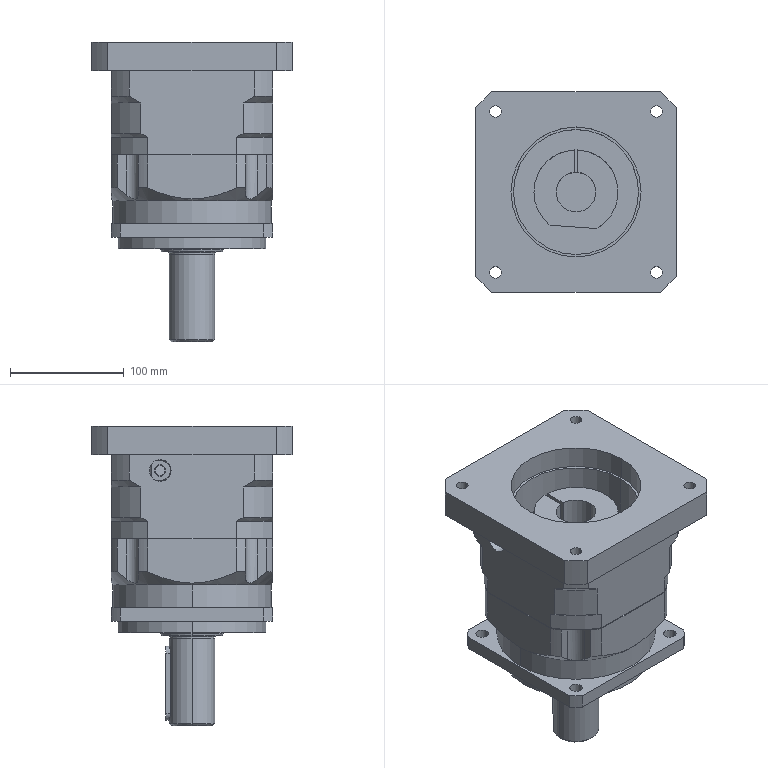Part | STEP file | PN_0046_default | 1 solid | 589 faces | box 176 x 176 x 263.5 mm | volume 3077737 mm3 | plane 360 | cylinder 109 | spline 86 | cone 32 | torus 2 | commonest cylinder face diameters 162 x12 7.42 x8 10.2 x8 11 x8 5.32 x7 20 x4